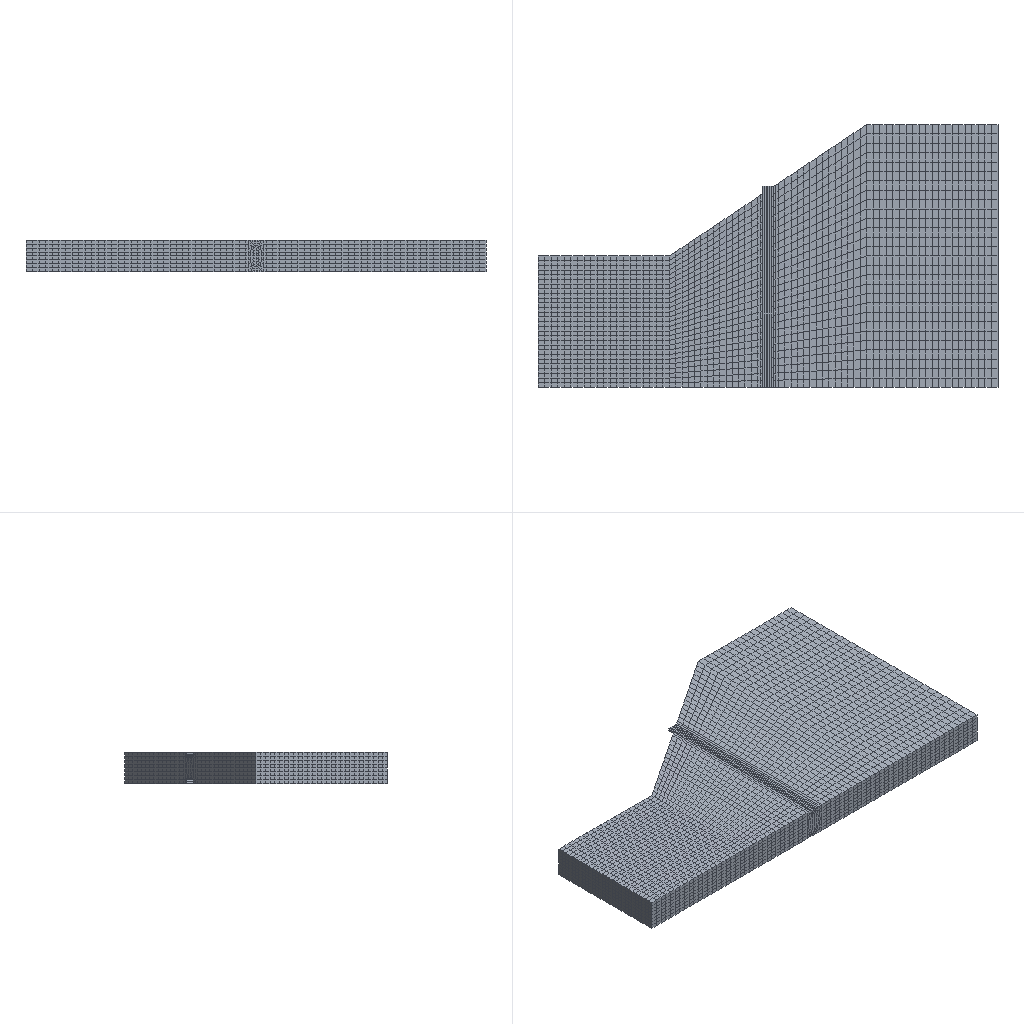Simulation study | abaqus
Set-up summary:
category,name,step,type,value,unit,region
solver,abaqus,,Abaqus/CAE 2024
units,unstated,,unstated,E=3e+07 density=2.4 (no match)
analysis,load,,static,time_period=1
mesh,nodes,,,21337
mesh,elements,,,17776
element_type,C3D8,,,17776
material,pile,,E,3e+07
material,pile,,nu,0.2
material,pile,,density,2.4
material,soil,,E,200000
material,soil,,nu,0.25
material,soil,,density,2
material,soil,,behaviors,plastic; mohr coulomb; mohr coulomb hardening
section,pile,,solid section,,,_PickedSet2
section,soil,,solid section,,,_PickedSet6
load,Load-1,load,gravity,"10 [dir=(0, -1, 0)]",,_PickedSet40
bc,BC-1,initial,fixed,"[dofs=rx,ry,rz,x,y,z n=6]",,_PickedSet19
bc,BC-2,initial,fixed,[dofs=x],,_PickedSet20
bc,BC-3,initial,fixed,[dofs=z],,_PickedSet37
contact,Constraint-1,initial,tie,,,_PickedSurf34 / _PickedSurf33
contact,Constraint-2,initial,tie,,,_PickedSurf36 / _PickedSurf35
contact,Int-1,initial,contact pair surface to surface,interaction=IntProp-1; friction=0.3; behavior=hard,,_PickedSurf39 / m_Surf-7
Abaqus input file, long lists of numbers shortened:
*Heading
** Job name: deck Model name: Model-1
** Generated by: Abaqus/CAE 2024
*Preprint, echo=NO, model=NO, history=NO, contact=NO
**
** PARTS
**
*Part, name=pile
*Node
      1, -0.4,          -5.,           0.
      2,  0.4,          -5.,           0.
** (1006 more lines like these left out)
*Element, type=C3D8
  1, 135, 133,  16,  15, 631, 629, 252, 253
  2, 135, 136, 134, 133, 631, 632, 630, 629
** (638 more lines like these left out)
*Nset, nset=_PickedSet2, internal, generate
    1,  1008,     1
*Elset, elset=_PickedSet2, internal, generate
   1,  640,    1
** Section: pile
*Solid Section, elset=_PickedSet2, material=pile
,
*End Part
**
*Part, name=soil
*Node
      1,         17.5,          15.,   1.2
      2,         17.5,          15.,           2.
** (20327 more lines like these left out)
*Element, type=C3D8
  1, 1164, 1165, 7401, 7319,   45,   44, 1003, 1002
  2, 1165, 1166, 7402, 7401,   44,   43, 1004, 1003
** (17134 more lines like these left out)
*Nset, nset=_PickedSet6, internal, generate
     1,  20329,      1
*Elset, elset=_PickedSet6, internal, generate
     1,  17136,      1
*Nset, nset=soil, generate
     1,  20329,      1
*Elset, elset=soil, generate
     1,  17136,      1
** Section: soil
*Solid Section, elset=_PickedSet6, material=soil
,
*End Part
**
**
** ASSEMBLY
**
*Assembly, name=Assembly
**
*Instance, name=pile-1, part=pile
        17.5,         15.3,           5.
        17.5,         15.3,           5., 18.5,         15.3,           5., 90.
*End Instance
**
*Instance, name=soil-1, part=soil
*End Instance
**
*Nset, nset=_PickedSet19, internal, instance=pile-1
   3,   4,   7,   8,  59,  60,  61,  62,  63,  64,  65,  66,  67,  68,  69,  70
 121, 122, 123, 124, 125, 126, 127, 128, 129, 130, 131, 132, 143, 144, 145, 146
** (1 more lines like these left out)
*Nset, nset=_PickedSet19, internal, instance=soil-1
    3,    4,    8,    9,   10,   11,   14,   15,   17,   20,   21,   23,   24,   25,   26,   31
   32,   33,   37,   39,   40,  106,  107,  108,  109,  110,  111,  112,  113,  114,  200,  201
** (42 more lines like these left out)
*Elset, elset=_PickedSet19, internal, instance=pile-1
 305, 306, 307, 308, 309, 310, 311, 312, 313, 314, 315, 316, 317, 318, 319, 320
 625, 626, 627, 628, 629, 630, 631, 632, 633, 634, 635, 636, 637, 638, 639, 640
*Elset, elset=_PickedSet19, internal, instance=soil-1
   169,   183,   197,   224,   238,   252,   266,   280,   294,   308,   322,   336,   407,   421,   422,   423
   463,   477,   478,   479,   588,   589,   590,   591,   631,   632,   633,   673,   674,   675,   841,   855
** (37 more lines like these left out)
*Nset, nset=_PickedSet20, internal, instance=soil-1
   25,   26,   28,   29,   39,   40,   41,   42,  432,  433,  434,  435,  436,  437,  438,  484
  485,  486,  487,  488,  489,  490,  510,  511,  512,  513,  514,  515,  516,  517,  518,  519
** (31 more lines like these left out)
*Elset, elset=_PickedSet20, internal, instance=soil-1
  1581,  1582,  1583,  1584,  1585,  1586,  1587,  1588,  1741,  1742,  1743,  1744,  1745,  1746,  1747,  1748
  1901,  1902,  1903,  1904,  1905,  1906,  1907,  1908,  2061,  2062,  2063,  2064,  2065,  2066,  2067,  2068
** (26 more lines like these left out)
*Nset, nset=_PickedSet37, internal, instance=pile-1
   1,   2,   3,   4,   5,   6,   7,   8,   9,  10,  11,  12,  13,  21,  22,  23
  24,  25,  26,  27,  28,  29,  30,  31,  32,  33,  34,  35,  36,  37,  38,  39
** (17 more lines like these left out)
*Nset, nset=_PickedSet37, internal, instance=soil-1
    5,    6,    8,   10,   13,   14,   15,   16,   17,   18,   19,   20,   23,   24,   25,   26
   27,   28,   29,   30,   31,   32,   33,   34,   35,   36,   37,   38,   39,   40,   41,   42
** (267 more lines like these left out)
*Elset, elset=_PickedSet37, internal, instance=pile-1
   3,   4,   6,   7,   8,  16,  19,  20,  22,  23,  24,  32,  35,  36,  38,  39
  40,  48,  51,  52,  54,  55,  56,  64,  67,  68,  70,  71,  72,  80,  83,  84
** (13 more lines like these left out)
*Elset, elset=_PickedSet37, internal, instance=soil-1
   337,   338,   339,   340,   341,   342,   343,   344,   345,   346,   347,   348,   349,   350,   351,   352
   353,   354,   355,   356,   357,   358,   359,   360,   361,   362,   363,   364,   407,   408,   409,   410
** (250 more lines like these left out)
*Nset, nset=_PickedSet40, internal, instance=pile-1, generate
    1,  1008,     1
*Nset, nset=_PickedSet40, internal, instance=soil-1, generate
     1,  20329,      1
*Elset, elset=_PickedSet40, internal, instance=pile-1, generate
   1,  640,    1
*Elset, elset=_PickedSet40, internal, instance=soil-1, generate
     1,  17136,      1
*Elset, elset=_m_Surf-7_S5, internal, instance=pile-1
   1,  15,  16,  17,  31,  32,  33,  47,  48,  49,  63,  64,  65,  79,  80,  81
  95,  96,  97, 111, 112, 113, 127, 128, 129, 143, 144, 145, 159, 160, 161, 175
** (6 more lines like these left out)
*Elset, elset=_m_Surf-7_S4, internal, instance=pile-1
   4,   5,  12,  13,  14,  20,  21,  28,  29,  30,  36,  37,  44,  45,  46,  52
  53,  60,  61,  62,  68,  69,  76,  77,  78,  84,  85,  92,  93,  94, 100, 101
** (11 more lines like these left out)
*Surface, type=ELEMENT, name=m_Surf-7
_m_Surf-7_S5, S5
_m_Surf-7_S4, S4
*Elset, elset=__PickedSurf33_S2, internal, instance=pile-1, generate
 625,  640,    1
*Surface, type=ELEMENT, name=_PickedSurf33, internal
__PickedSurf33_S2, S2
*Elset, elset=__PickedSurf34_S3, internal, instance=soil-1
  169,  183,  197,  407, 9073
*Elset, elset=__PickedSurf34_S4, internal, instance=soil-1
  224,  238,  252,  266,  280,  294,  308,  322,  336, 9072, 9156, 9170, 9184, 9324, 9338, 9352
 9366, 9380, 9394, 9408, 9422, 9436, 9492, 9506, 9520
*Elset, elset=__PickedSurf34_S2, internal, instance=soil-1
 421, 422, 423, 463
*Surface, type=ELEMENT, name=_PickedSurf34, internal
__PickedSurf34_S3, S3
__PickedSurf34_S4, S4
__PickedSurf34_S2, S2
*Elset, elset=__PickedSurf35_S2, internal, instance=pile-1, generate
 305,  320,    1
*Surface, type=ELEMENT, name=_PickedSurf35, internal
__PickedSurf35_S2, S2
*Elset, elset=__PickedSurf36_S3, internal, instance=soil-1
  477,  478,  479,  589,  590,  591,  631,  632,  633,  673,  674,  675,  953, 1009, 1010, 1011
 1219, 1220, 1221, 1261, 1262, 1263, 1303, 1304, 1305, 1387, 1401, 1415
*Elset, elset=__PickedSurf36_S4, internal, instance=soil-1
  588, 1008
*Elset, elset=__PickedSurf36_S2, internal, instance=soil-1
 841, 855, 856, 857
*Surface, type=ELEMENT, name=_PickedSurf36, internal
__PickedSurf36_S3, S3
__PickedSurf36_S4, S4
__PickedSurf36_S2, S2
*Elset, elset=__PickedSurf39_S4, internal, instance=soil-1
  169,  170,  171,  172,  173,  174,  175,  176,  177,  178,  179,  180,  181,  182,  183,  184
  185,  186,  187,  188,  189,  190,  191,  192,  193,  194,  195,  196,  197,  198,  199,  200
** (8 more lines like these left out)
*Elset, elset=__PickedSurf39_S3, internal, instance=soil-1
  127,  128,  129,  130,  131,  132,  133,  134,  135,  136,  137,  138,  139,  140,  141,  142
  143,  144,  145,  146,  147,  148,  149,  150,  151,  152,  153,  154,  155,  156,  157,  158
** (9 more lines like these left out)
*Elset, elset=__PickedSurf39_S2, internal, instance=soil-1
 407, 408, 409, 410, 411, 412, 413, 414, 415, 416, 417, 418, 419, 420, 477, 478
 479, 480, 481, 482, 483, 484, 485, 486, 487, 488, 489, 490, 491, 492, 493, 494
** (6 more lines like these left out)
*Surface, type=ELEMENT, name=_PickedSurf39, internal
__PickedSurf39_S4, S4
__PickedSurf39_S3, S3
__PickedSurf39_S2, S2
** Constraint: Constraint-1
*Tie, name=Constraint-1, adjust=yes
_PickedSurf34, _PickedSurf33
** Constraint: Constraint-2
*Tie, name=Constraint-2, adjust=yes
_PickedSurf36, _PickedSurf35
*End Assembly
**
** MATERIALS
**
*Material, name=pile
*Density
 2.4,
*Elastic
 3e+07, 0.2
*Material, name=soil
*Density
2.,
*Elastic
200000., 0.25
*Mohr Coulomb
 36.052,0.
*Mohr Coulomb Hardening
20.,0.
**
** INTERACTION PROPERTIES
**
*Surface Interaction, name=IntProp-1
1.,
*Friction, slip tolerance=0.005
 0.3,
*Surface Behavior, pressure-overclosure=HARD
**
** BOUNDARY CONDITIONS
**
** Name: BC-1 Type: Displacement/Rotation
*Boundary
_PickedSet19, 1, 1
_PickedSet19, 2, 2
_PickedSet19, 3, 3
_PickedSet19, 4, 4
_PickedSet19, 5, 5
_PickedSet19, 6, 6
** Name: BC-2 Type: Displacement/Rotation
*Boundary
_PickedSet20, 1, 1
** Name: BC-3 Type: Displacement/Rotation
*Boundary
_PickedSet37, 3, 3
**
** INTERACTIONS
**
** Interaction: Int-1
*Contact Pair, interaction=IntProp-1, type=SURFACE TO SURFACE, adjust=0.02
_PickedSurf39, m_Surf-7
** ----------------------------------------------------------------
**
** STEP: load
**
*Step, name=load, nlgeom=NO, unsymm=YES
*Static
0.01, 1., 1e-05, 1.
**
** LOADS
**
** Name: Load-1   Type: Gravity
*Dload
_PickedSet40, GRAV, 10., 0., -1., 0.
**
** OUTPUT REQUESTS
**
*Restart, write, frequency=0
**
** FIELD OUTPUT: F-Output-1
**
*Output, field, variable=PRESELECT
**
** HISTORY OUTPUT: H-Output-1
**
*Output, history, variable=PRESELECT
*End Step
Results summary:
result,odb.job_status,,,JOB_STATUS_COMPLETED_SUCCESSFULLY,"consistent, unstated (Abaqus has no unit system)"
result,steps[0].procedure,load,,*STATIC,"consistent, unstated (Abaqus has no unit system)"
result,steps[0].time_period,load,,1,"consistent, unstated (Abaqus has no unit system)"
result,steps[0].n_frames,load,,12,"consistent, unstated (Abaqus has no unit system)"
result,steps[0].last_frame.id,load,,11,"consistent, unstated (Abaqus has no unit system)"
result,steps[0].last_frame.value,load,,1,"consistent, unstated (Abaqus has no unit system)"
result,steps[0].last_frame.description,load,,Increment     11: Step Time =    1.000,"consistent, unstated (Abaqus has no unit system)"
result,steps[0].completed,load,,True,"consistent, unstated (Abaqus has no unit system)"
result,steps[0].max_U_magnitude,load,,0.0165,"consistent, unstated (Abaqus has no unit system)"
result,steps[0].max_S_mises,load,,4209.6,"consistent, unstated (Abaqus has no unit system)"
result,steps[0].RF_sum[1],load,,0.0005622,"consistent, unstated (Abaqus has no unit system)"
result,steps[0].RF_sum[2],load,,25232.9,"consistent, unstated (Abaqus has no unit system)"
result,steps[0].RF_sum[3],load,,0.003748,"consistent, unstated (Abaqus has no unit system)"